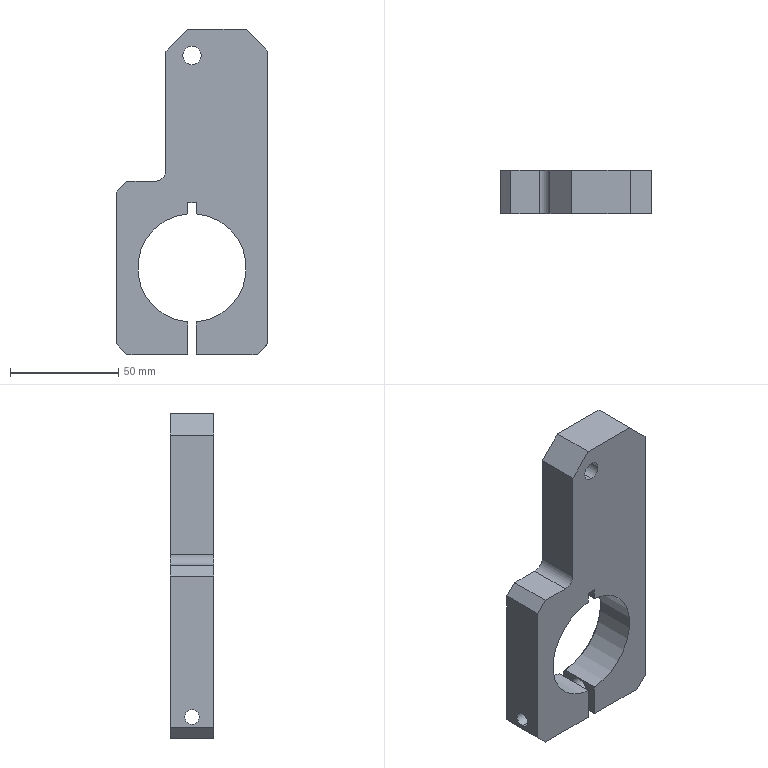Part | STEP file | 0229_217_Arm | 1 solid | 33 faces | box 70 x 20 x 150 mm | volume 127979 mm3 | plane 20 | cylinder 11 | cone 2 | commonest cylinder face diameters 6.8 x2 8.5 x2 9 x2 14 x2 50 x2 10 x1